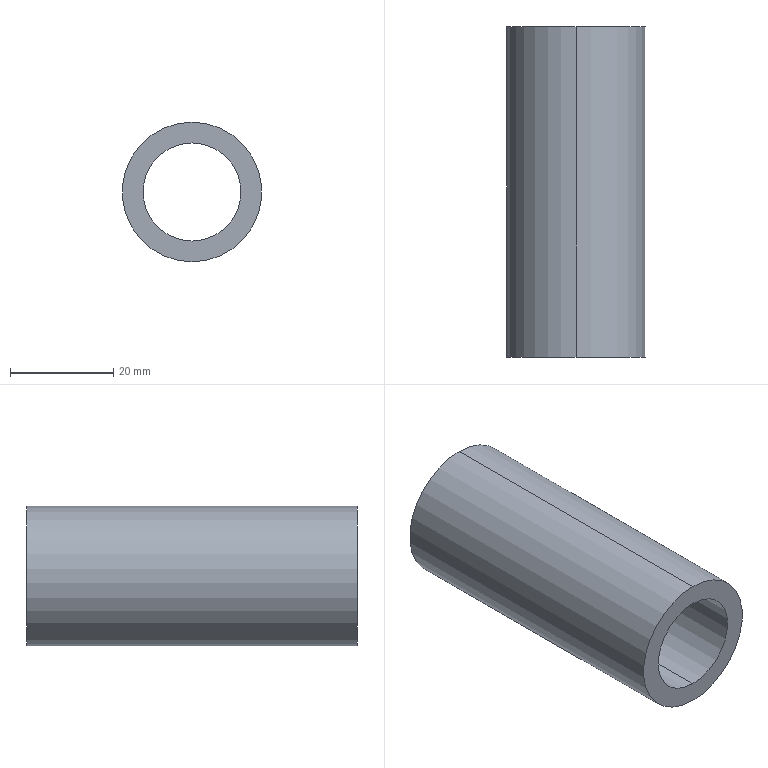Part | SolidWorks | features Extrusion 1 | 1 solid | 6 faces | box 27 x 64 x 27 mm | volume 18498 mm3 | cylinder 4 | plane 2 | commonest cylinder face diameters 19 x2 27 x2
STEP:
#1=CARTESIAN_POINT('',(0.,64.,-9.5));
#2=VERTEX_POINT('',#1);
#3=CARTESIAN_POINT('',(0.,64.,9.5));
#4=VERTEX_POINT('',#3);
#5=CARTESIAN_POINT('',(0.,64.,0.));
#6=DIRECTION('',(0.,1.,0.));
#7=DIRECTION('',(0.,0.,1.));
#8=AXIS2_PLACEMENT_3D('',#5,#6,#7);
#9=CIRCLE('',#8,9.5);
#10=EDGE_CURVE('',#2,#4,#9,.T.);
#11=ORIENTED_EDGE('',*,*,#10,.T.);
#12=CARTESIAN_POINT('',(0.,0.,9.5));
#13=VERTEX_POINT('',#12);
#14=CARTESIAN_POINT('',(0.,64.,9.5));
#15=DIRECTION('',(0.,-1.,0.));
#16=VECTOR('',#15,1000.);
#17=LINE('',#14,#16);
#18=EDGE_CURVE('',#4,#13,#17,.T.);
#19=ORIENTED_EDGE('',*,*,#18,.T.);
#20=CARTESIAN_POINT('',(0.,0.,-9.5));
#21=VERTEX_POINT('',#20);
#22=CARTESIAN_POINT('',(0.,0.,0.));
#23=DIRECTION('',(0.,1.,0.));
#24=DIRECTION('',(0.,0.,1.));
#25=AXIS2_PLACEMENT_3D('',#22,#23,#24);
#26=CIRCLE('',#25,9.5);
#27=EDGE_CURVE('',#21,#13,#26,.T.);
#28=ORIENTED_EDGE('',*,*,#27,.F.);
#29=CARTESIAN_POINT('',(0.,64.,-9.5));
#30=DIRECTION('',(0.,-1.,0.));
#31=VECTOR('',#30,1000.);
#32=LINE('',#29,#31);
#33=EDGE_CURVE('',#2,#21,#32,.T.);
#34=ORIENTED_EDGE('',*,*,#33,.F.);
#35=EDGE_LOOP('',(#11,#19,#28,#34));
#36=FACE_OUTER_BOUND('',#35,.T.);
#37=CARTESIAN_POINT('',(0.,64.,0.));
#38=DIRECTION('',(0.,-1.,0.));
#39=DIRECTION('',(0.,0.,-1.));
#40=AXIS2_PLACEMENT_3D('',#37,#38,#39);
#41=CYLINDRICAL_SURFACE('',#40,9.5);
#42=ADVANCED_FACE('',(#36),#41,.F.);
#43=CARTESIAN_POINT('',(0.,64.,13.5));
#44=VERTEX_POINT('',#43);
#45=CARTESIAN_POINT('',(0.,64.,-13.5));
#46=VERTEX_POINT('',#45);
#47=CARTESIAN_POINT('',(0.,64.,0.));
#48=DIRECTION('',(0.,1.,0.));
#49=DIRECTION('',(0.,0.,1.));
#50=AXIS2_PLACEMENT_3D('',#47,#48,#49);
#51=CIRCLE('',#50,13.5);
#52=EDGE_CURVE('',#44,#46,#51,.T.);
#53=ORIENTED_EDGE('',*,*,#52,.F.);
#54=CARTESIAN_POINT('',(0.,0.,13.5));
#55=VERTEX_POINT('',#54);
#56=CARTESIAN_POINT('',(0.,64.,13.5));
#57=DIRECTION('',(0.,-1.,0.));
#58=VECTOR('',#57,1000.);
#59=LINE('',#56,#58);
#60=EDGE_CURVE('',#44,#55,#59,.T.);
#61=ORIENTED_EDGE('',*,*,#60,.T.);
#62=CARTESIAN_POINT('',(0.,0.,-13.5));
#63=VERTEX_POINT('',#62);
#64=CARTESIAN_POINT('',(0.,0.,0.));
#65=DIRECTION('',(0.,1.,0.));
#66=DIRECTION('',(0.,0.,1.));
#67=AXIS2_PLACEMENT_3D('',#64,#65,#66);
#68=CIRCLE('',#67,13.5);
#69=EDGE_CURVE('',#55,#63,#68,.T.);
#70=ORIENTED_EDGE('',*,*,#69,.T.);
#71=CARTESIAN_POINT('',(0.,64.,-13.5));
#72=DIRECTION('',(0.,-1.,0.));
#73=VECTOR('',#72,1000.);
#74=LINE('',#71,#73);
#75=EDGE_CURVE('',#46,#63,#74,.T.);
#76=ORIENTED_EDGE('',*,*,#75,.F.);
#77=EDGE_LOOP('',(#53,#61,#70,#76));
#78=FACE_OUTER_BOUND('',#77,.T.);
#79=CARTESIAN_POINT('',(0.,64.,0.));
#80=DIRECTION('',(0.,-1.,0.));
#81=DIRECTION('',(0.,0.,-1.));
#82=AXIS2_PLACEMENT_3D('',#79,#80,#81);
#83=CYLINDRICAL_SURFACE('',#82,13.5);
#84=ADVANCED_FACE('',(#78),#83,.T.);
#85=CARTESIAN_POINT('',(0.,64.,0.));
#86=DIRECTION('',(0.,1.,0.));
#87=DIRECTION('',(0.,0.,1.));
#88=AXIS2_PLACEMENT_3D('',#85,#86,#87);
#89=CIRCLE('',#88,13.5);
#90=EDGE_CURVE('',#46,#44,#89,.T.);
#91=ORIENTED_EDGE('',*,*,#90,.T.);
#92=ORIENTED_EDGE('',*,*,#52,.T.);
#93=EDGE_LOOP('',(#91,#92));
#94=FACE_OUTER_BOUND('',#93,.T.);
#95=ORIENTED_EDGE('',*,*,#10,.F.);
#96=CARTESIAN_POINT('',(0.,64.,0.));
#97=DIRECTION('',(0.,1.,0.));
#98=DIRECTION('',(0.,0.,1.));
#99=AXIS2_PLACEMENT_3D('',#96,#97,#98);
#100=CIRCLE('',#99,9.5);
#101=EDGE_CURVE('',#4,#2,#100,.T.);
#102=ORIENTED_EDGE('',*,*,#101,.F.);
#103=EDGE_LOOP('',(#95,#102));
#104=FACE_BOUND('',#103,.T.);
#105=CARTESIAN_POINT('',(0.,64.,0.));
#106=DIRECTION('',(0.,1.,0.));
#107=DIRECTION('',(0.,0.,1.));
#108=AXIS2_PLACEMENT_3D('',#105,#106,#107);
#109=PLANE('',#108);
#110=ADVANCED_FACE('',(#94,#104),#109,.T.);
#111=CARTESIAN_POINT('',(0.,0.,0.));
#112=DIRECTION('',(0.,1.,0.));
#113=DIRECTION('',(0.,0.,1.));
#114=AXIS2_PLACEMENT_3D('',#111,#112,#113);
#115=CIRCLE('',#114,13.5);
#116=EDGE_CURVE('',#63,#55,#115,.T.);
#117=ORIENTED_EDGE('',*,*,#116,.F.);
#118=ORIENTED_EDGE('',*,*,#69,.F.);
#119=EDGE_LOOP('',(#117,#118));
#120=FACE_OUTER_BOUND('',#119,.T.);
#121=ORIENTED_EDGE('',*,*,#27,.T.);
#122=CARTESIAN_POINT('',(0.,0.,0.));
#123=DIRECTION('',(0.,1.,0.));
#124=DIRECTION('',(0.,0.,1.));
#125=AXIS2_PLACEMENT_3D('',#122,#123,#124);
#126=CIRCLE('',#125,9.5);
#127=EDGE_CURVE('',#13,#21,#126,.T.);
#128=ORIENTED_EDGE('',*,*,#127,.T.);
#129=EDGE_LOOP('',(#121,#128));
#130=FACE_BOUND('',#129,.T.);
#131=CARTESIAN_POINT('',(0.,0.,0.));
#132=DIRECTION('',(0.,1.,0.));
#133=DIRECTION('',(0.,0.,1.));
#134=AXIS2_PLACEMENT_3D('',#131,#132,#133);
#135=PLANE('',#134);
#136=ADVANCED_FACE('',(#120,#130),#135,.F.);
#137=ORIENTED_EDGE('',*,*,#60,.F.);
#138=ORIENTED_EDGE('',*,*,#90,.F.);
#139=ORIENTED_EDGE('',*,*,#75,.T.);
#140=ORIENTED_EDGE('',*,*,#116,.T.);
#141=EDGE_LOOP('',(#137,#138,#139,#140));
#142=FACE_OUTER_BOUND('',#141,.T.);
#143=CARTESIAN_POINT('',(0.,64.,0.));
#144=DIRECTION('',(0.,-1.,0.));
#145=DIRECTION('',(0.,0.,-1.));
#146=AXIS2_PLACEMENT_3D('',#143,#144,#145);
#147=CYLINDRICAL_SURFACE('',#146,13.5);
#148=ADVANCED_FACE('',(#142),#147,.T.);
#149=ORIENTED_EDGE('',*,*,#18,.F.);
#150=ORIENTED_EDGE('',*,*,#101,.T.);
#151=ORIENTED_EDGE('',*,*,#33,.T.);
#152=ORIENTED_EDGE('',*,*,#127,.F.);
#153=EDGE_LOOP('',(#149,#150,#151,#152));
#154=FACE_OUTER_BOUND('',#153,.T.);
#155=CARTESIAN_POINT('',(0.,64.,0.));
#156=DIRECTION('',(0.,-1.,0.));
#157=DIRECTION('',(0.,0.,-1.));
#158=AXIS2_PLACEMENT_3D('',#155,#156,#157);
#159=CYLINDRICAL_SURFACE('',#158,9.5);
#160=ADVANCED_FACE('',(#154),#159,.F.);
#161=CLOSED_SHELL('',(#42,#84,#110,#136,#148,#160));
#162=MANIFOLD_SOLID_BREP('',#161);
#163=CARTESIAN_POINT('',(0.,0.,0.));
#164=DIRECTION('',(0.,0.,1.));
#165=DIRECTION('',(1.,0.,0.));
#166=AXIS2_PLACEMENT_3D('',#163,#164,#165);
#167=(LENGTH_UNIT()NAMED_UNIT(*)SI_UNIT(.MILLI.,.METRE.));
#168=UNCERTAINTY_MEASURE_WITH_UNIT(LENGTH_MEASURE(0.00001),#167,'','');
#169=(NAMED_UNIT(*)PLANE_ANGLE_UNIT()SI_UNIT($,.RADIAN.));
#170=(NAMED_UNIT(*)SI_UNIT($,.STERADIAN.)SOLID_ANGLE_UNIT());
#171=(GEOMETRIC_REPRESENTATION_CONTEXT(3)GLOBAL_UNCERTAINTY_ASSIGNED_CONTEXT((#168))GLOBAL_UNIT_ASSIGNED_CONTEXT((#167,#169,#170))REPRESENTATION_CONTEXT('',''));
#172=ADVANCED_BREP_SHAPE_REPRESENTATION('',(#162,#166),#171);